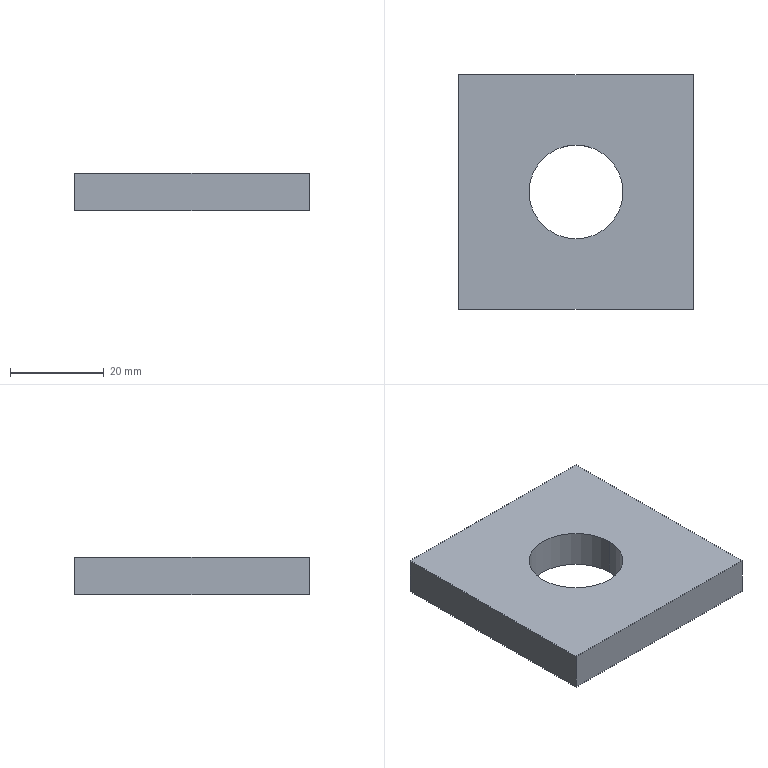Part | STEP file | 立柱底Plate方形垫片 | 1 solid | 8 faces | box 50 x 50 x 8 mm | volume 17487 mm3 | plane 6 | cylinder 2 | commonest cylinder face diameters 20 x2
STEP:
#1=CARTESIAN_POINT('',(0.,0.,0.));
#2=DIRECTION('',(0.,0.,1.));
#3=DIRECTION('',(1.,0.,0.));
#4=AXIS2_PLACEMENT_3D('',#1,#2,#3);
#5=CARTESIAN_POINT('',(-10.,0.,8.));
#6=VERTEX_POINT('',#5);
#7=CARTESIAN_POINT('',(-10.,0.,0.));
#8=VERTEX_POINT('',#7);
#9=CARTESIAN_POINT('',(-10.,0.,8.));
#10=DIRECTION('',(0.,0.,-1.));
#11=VECTOR('',#10,1.);
#12=LINE('',#9,#11);
#13=CARTESIAN_POINT('',(0.,0.,8.));
#14=DIRECTION('',(0.,0.,-1.));
#15=DIRECTION('',(-1.,0.,0.));
#16=AXIS2_PLACEMENT_3D('',#13,#14,#15);
#17=CYLINDRICAL_SURFACE('',#16,10.);
#18=CARTESIAN_POINT('',(6.283,0.));
#19=DIRECTION('',(0.,1.));
#20=VECTOR('',#19,1.);
#21=LINE('',#18,#20);
#22=(GEOMETRIC_REPRESENTATION_CONTEXT(2)PARAMETRIC_REPRESENTATION_CONTEXT()REPRESENTATION_CONTEXT('',''));
#23=DEFINITIONAL_REPRESENTATION('',(#21),#22);
#24=PCURVE('',#17,#23);
#25=CARTESIAN_POINT('',(0.,0.,8.));
#26=DIRECTION('',(0.,0.,-1.));
#27=DIRECTION('',(-1.,0.,0.));
#28=AXIS2_PLACEMENT_3D('',#25,#26,#27);
#29=CYLINDRICAL_SURFACE('',#28,10.);
#30=CARTESIAN_POINT('',(0.,0.));
#31=DIRECTION('',(0.,1.));
#32=VECTOR('',#31,1.);
#33=LINE('',#30,#32);
#34=(GEOMETRIC_REPRESENTATION_CONTEXT(2)PARAMETRIC_REPRESENTATION_CONTEXT()REPRESENTATION_CONTEXT('',''));
#35=DEFINITIONAL_REPRESENTATION('',(#33),#34);
#36=PCURVE('',#29,#35);
#37=SURFACE_CURVE('',#12,(#24,#36),.PCURVE_S1.);
#38=EDGE_CURVE('',#6,#8,#37,.T.);
#39=ORIENTED_EDGE('',*,*,#38,.T.);
#40=CARTESIAN_POINT('',(10.,0.,0.));
#41=VERTEX_POINT('',#40);
#42=CARTESIAN_POINT('',(0.,0.,0.));
#43=DIRECTION('',(0.,0.,1.));
#44=DIRECTION('',(1.,0.,0.));
#45=AXIS2_PLACEMENT_3D('',#42,#43,#44);
#46=CIRCLE('',#45,10.);
#47=CARTESIAN_POINT('',(9.425,8.));
#48=DIRECTION('',(-1.,0.));
#49=VECTOR('',#48,1.);
#50=LINE('',#47,#49);
#51=(GEOMETRIC_REPRESENTATION_CONTEXT(2)PARAMETRIC_REPRESENTATION_CONTEXT()REPRESENTATION_CONTEXT('',''));
#52=DEFINITIONAL_REPRESENTATION('',(#50),#51);
#53=PCURVE('',#17,#52);
#54=CARTESIAN_POINT('',(0.,0.,0.));
#55=DIRECTION('',(0.,0.,1.));
#56=DIRECTION('',(1.,0.,0.));
#57=AXIS2_PLACEMENT_3D('',#54,#55,#56);
#58=PLANE('',#57);
#59=CARTESIAN_POINT('',(0.,0.));
#60=DIRECTION('',(1.,0.));
#61=AXIS2_PLACEMENT_2D('',#59,#60);
#62=CIRCLE('',#61,10.);
#63=(GEOMETRIC_REPRESENTATION_CONTEXT(2)PARAMETRIC_REPRESENTATION_CONTEXT()REPRESENTATION_CONTEXT('',''));
#64=DEFINITIONAL_REPRESENTATION('',(#62),#63);
#65=PCURVE('',#58,#64);
#66=SURFACE_CURVE('',#46,(#53,#65),.PCURVE_S1.);
#67=EDGE_CURVE('',#8,#41,#66,.T.);
#68=ORIENTED_EDGE('',*,*,#67,.T.);
#69=CARTESIAN_POINT('',(10.,0.,8.));
#70=VERTEX_POINT('',#69);
#71=CARTESIAN_POINT('',(10.,0.,8.));
#72=DIRECTION('',(0.,0.,-1.));
#73=VECTOR('',#72,1.);
#74=LINE('',#71,#73);
#75=CARTESIAN_POINT('',(3.142,0.));
#76=DIRECTION('',(0.,1.));
#77=VECTOR('',#76,1.);
#78=LINE('',#75,#77);
#79=(GEOMETRIC_REPRESENTATION_CONTEXT(2)PARAMETRIC_REPRESENTATION_CONTEXT()REPRESENTATION_CONTEXT('',''));
#80=DEFINITIONAL_REPRESENTATION('',(#78),#79);
#81=PCURVE('',#17,#80);
#82=CARTESIAN_POINT('',(3.142,0.));
#83=DIRECTION('',(0.,1.));
#84=VECTOR('',#83,1.);
#85=LINE('',#82,#84);
#86=(GEOMETRIC_REPRESENTATION_CONTEXT(2)PARAMETRIC_REPRESENTATION_CONTEXT()REPRESENTATION_CONTEXT('',''));
#87=DEFINITIONAL_REPRESENTATION('',(#85),#86);
#88=PCURVE('',#29,#87);
#89=SURFACE_CURVE('',#74,(#81,#88),.PCURVE_S1.);
#90=EDGE_CURVE('',#70,#41,#89,.T.);
#91=ORIENTED_EDGE('',*,*,#90,.F.);
#92=CARTESIAN_POINT('',(0.,0.,8.));
#93=DIRECTION('',(0.,0.,1.));
#94=DIRECTION('',(1.,0.,0.));
#95=AXIS2_PLACEMENT_3D('',#92,#93,#94);
#96=CIRCLE('',#95,10.);
#97=CARTESIAN_POINT('',(9.425,0.));
#98=DIRECTION('',(-1.,0.));
#99=VECTOR('',#98,1.);
#100=LINE('',#97,#99);
#101=(GEOMETRIC_REPRESENTATION_CONTEXT(2)PARAMETRIC_REPRESENTATION_CONTEXT()REPRESENTATION_CONTEXT('',''));
#102=DEFINITIONAL_REPRESENTATION('',(#100),#101);
#103=PCURVE('',#17,#102);
#104=CARTESIAN_POINT('',(0.,0.,8.));
#105=DIRECTION('',(0.,0.,1.));
#106=DIRECTION('',(1.,0.,0.));
#107=AXIS2_PLACEMENT_3D('',#104,#105,#106);
#108=PLANE('',#107);
#109=CARTESIAN_POINT('',(0.,0.));
#110=DIRECTION('',(1.,0.));
#111=AXIS2_PLACEMENT_2D('',#109,#110);
#112=CIRCLE('',#111,10.);
#113=(GEOMETRIC_REPRESENTATION_CONTEXT(2)PARAMETRIC_REPRESENTATION_CONTEXT()REPRESENTATION_CONTEXT('',''));
#114=DEFINITIONAL_REPRESENTATION('',(#112),#113);
#115=PCURVE('',#108,#114);
#116=SURFACE_CURVE('',#96,(#103,#115),.PCURVE_S1.);
#117=EDGE_CURVE('',#6,#70,#116,.T.);
#118=ORIENTED_EDGE('',*,*,#117,.F.);
#119=EDGE_LOOP('',(#39,#68,#91,#118));
#120=FACE_BOUND('',#119,.F.);
#121=ADVANCED_FACE('',(#120),#17,.F.);
#122=CARTESIAN_POINT('',(25.,-25.,8.));
#123=VERTEX_POINT('',#122);
#124=CARTESIAN_POINT('',(25.,25.,8.));
#125=VERTEX_POINT('',#124);
#126=CARTESIAN_POINT('',(25.,25.,8.));
#127=DIRECTION('',(0.,1.,0.));
#128=VECTOR('',#127,1.);
#129=LINE('',#126,#128);
#130=CARTESIAN_POINT('',(25.,25.));
#131=DIRECTION('',(0.,1.));
#132=VECTOR('',#131,1.);
#133=LINE('',#130,#132);
#134=(GEOMETRIC_REPRESENTATION_CONTEXT(2)PARAMETRIC_REPRESENTATION_CONTEXT()REPRESENTATION_CONTEXT('',''));
#135=DEFINITIONAL_REPRESENTATION('',(#133),#134);
#136=PCURVE('',#108,#135);
#137=CARTESIAN_POINT('',(25.,25.,8.));
#138=DIRECTION('',(-1.,0.,0.));
#139=DIRECTION('',(0.,-1.,0.));
#140=AXIS2_PLACEMENT_3D('',#137,#138,#139);
#141=PLANE('',#140);
#142=CARTESIAN_POINT('',(0.,0.));
#143=DIRECTION('',(-1.,0.));
#144=VECTOR('',#143,1.);
#145=LINE('',#142,#144);
#146=(GEOMETRIC_REPRESENTATION_CONTEXT(2)PARAMETRIC_REPRESENTATION_CONTEXT()REPRESENTATION_CONTEXT('',''));
#147=DEFINITIONAL_REPRESENTATION('',(#145),#146);
#148=PCURVE('',#141,#147);
#149=SURFACE_CURVE('',#129,(#136,#148),.PCURVE_S1.);
#150=EDGE_CURVE('',#123,#125,#149,.T.);
#151=ORIENTED_EDGE('',*,*,#150,.T.);
#152=CARTESIAN_POINT('',(-25.,25.,8.));
#153=VERTEX_POINT('',#152);
#154=CARTESIAN_POINT('',(-25.,25.,8.));
#155=DIRECTION('',(-1.,0.,0.));
#156=VECTOR('',#155,1.);
#157=LINE('',#154,#156);
#158=CARTESIAN_POINT('',(-25.,25.));
#159=DIRECTION('',(-1.,0.));
#160=VECTOR('',#159,1.);
#161=LINE('',#158,#160);
#162=(GEOMETRIC_REPRESENTATION_CONTEXT(2)PARAMETRIC_REPRESENTATION_CONTEXT()REPRESENTATION_CONTEXT('',''));
#163=DEFINITIONAL_REPRESENTATION('',(#161),#162);
#164=PCURVE('',#108,#163);
#165=CARTESIAN_POINT('',(-25.,25.,8.));
#166=DIRECTION('',(0.,-1.,0.));
#167=DIRECTION('',(0.,0.,-1.));
#168=AXIS2_PLACEMENT_3D('',#165,#166,#167);
#169=PLANE('',#168);
#170=CARTESIAN_POINT('',(0.,0.));
#171=DIRECTION('',(0.,-1.));
#172=VECTOR('',#171,1.);
#173=LINE('',#170,#172);
#174=(GEOMETRIC_REPRESENTATION_CONTEXT(2)PARAMETRIC_REPRESENTATION_CONTEXT()REPRESENTATION_CONTEXT('',''));
#175=DEFINITIONAL_REPRESENTATION('',(#173),#174);
#176=PCURVE('',#169,#175);
#177=SURFACE_CURVE('',#157,(#164,#176),.PCURVE_S1.);
#178=EDGE_CURVE('',#125,#153,#177,.T.);
#179=ORIENTED_EDGE('',*,*,#178,.T.);
#180=CARTESIAN_POINT('',(-25.,-25.,8.));
#181=VERTEX_POINT('',#180);
#182=CARTESIAN_POINT('',(-25.,25.,8.));
#183=DIRECTION('',(0.,-1.,0.));
#184=VECTOR('',#183,1.);
#185=LINE('',#182,#184);
#186=CARTESIAN_POINT('',(-25.,25.));
#187=DIRECTION('',(0.,-1.));
#188=VECTOR('',#187,1.);
#189=LINE('',#186,#188);
#190=(GEOMETRIC_REPRESENTATION_CONTEXT(2)PARAMETRIC_REPRESENTATION_CONTEXT()REPRESENTATION_CONTEXT('',''));
#191=DEFINITIONAL_REPRESENTATION('',(#189),#190);
#192=PCURVE('',#108,#191);
#193=CARTESIAN_POINT('',(-25.,25.,8.));
#194=DIRECTION('',(1.,0.,0.));
#195=DIRECTION('',(0.,1.,0.));
#196=AXIS2_PLACEMENT_3D('',#193,#194,#195);
#197=PLANE('',#196);
#198=CARTESIAN_POINT('',(0.,0.));
#199=DIRECTION('',(-1.,0.));
#200=VECTOR('',#199,1.);
#201=LINE('',#198,#200);
#202=(GEOMETRIC_REPRESENTATION_CONTEXT(2)PARAMETRIC_REPRESENTATION_CONTEXT()REPRESENTATION_CONTEXT('',''));
#203=DEFINITIONAL_REPRESENTATION('',(#201),#202);
#204=PCURVE('',#197,#203);
#205=SURFACE_CURVE('',#185,(#192,#204),.PCURVE_S1.);
#206=EDGE_CURVE('',#153,#181,#205,.T.);
#207=ORIENTED_EDGE('',*,*,#206,.T.);
#208=CARTESIAN_POINT('',(-25.,-25.,8.));
#209=DIRECTION('',(1.,0.,0.));
#210=VECTOR('',#209,1.);
#211=LINE('',#208,#210);
#212=CARTESIAN_POINT('',(-25.,-25.));
#213=DIRECTION('',(1.,0.));
#214=VECTOR('',#213,1.);
#215=LINE('',#212,#214);
#216=(GEOMETRIC_REPRESENTATION_CONTEXT(2)PARAMETRIC_REPRESENTATION_CONTEXT()REPRESENTATION_CONTEXT('',''));
#217=DEFINITIONAL_REPRESENTATION('',(#215),#216);
#218=PCURVE('',#108,#217);
#219=CARTESIAN_POINT('',(-25.,-25.,8.));
#220=DIRECTION('',(0.,1.,0.));
#221=DIRECTION('',(0.,0.,1.));
#222=AXIS2_PLACEMENT_3D('',#219,#220,#221);
#223=PLANE('',#222);
#224=CARTESIAN_POINT('',(0.,0.));
#225=DIRECTION('',(0.,1.));
#226=VECTOR('',#225,1.);
#227=LINE('',#224,#226);
#228=(GEOMETRIC_REPRESENTATION_CONTEXT(2)PARAMETRIC_REPRESENTATION_CONTEXT()REPRESENTATION_CONTEXT('',''));
#229=DEFINITIONAL_REPRESENTATION('',(#227),#228);
#230=PCURVE('',#223,#229);
#231=SURFACE_CURVE('',#211,(#218,#230),.PCURVE_S1.);
#232=EDGE_CURVE('',#181,#123,#231,.T.);
#233=ORIENTED_EDGE('',*,*,#232,.T.);
#234=EDGE_LOOP('',(#151,#179,#207,#233));
#235=FACE_BOUND('',#234,.T.);
#236=ORIENTED_EDGE('',*,*,#117,.F.);
#237=CARTESIAN_POINT('',(0.,0.,8.));
#238=DIRECTION('',(0.,0.,1.));
#239=DIRECTION('',(1.,0.,0.));
#240=AXIS2_PLACEMENT_3D('',#237,#238,#239);
#241=CIRCLE('',#240,10.);
#242=CARTESIAN_POINT('',(0.,0.));
#243=DIRECTION('',(1.,0.));
#244=AXIS2_PLACEMENT_2D('',#242,#243);
#245=CIRCLE('',#244,10.);
#246=(GEOMETRIC_REPRESENTATION_CONTEXT(2)PARAMETRIC_REPRESENTATION_CONTEXT()REPRESENTATION_CONTEXT('',''));
#247=DEFINITIONAL_REPRESENTATION('',(#245),#246);
#248=PCURVE('',#108,#247);
#249=CARTESIAN_POINT('',(3.142,0.));
#250=DIRECTION('',(-1.,0.));
#251=VECTOR('',#250,1.);
#252=LINE('',#249,#251);
#253=(GEOMETRIC_REPRESENTATION_CONTEXT(2)PARAMETRIC_REPRESENTATION_CONTEXT()REPRESENTATION_CONTEXT('',''));
#254=DEFINITIONAL_REPRESENTATION('',(#252),#253);
#255=PCURVE('',#29,#254);
#256=SURFACE_CURVE('',#241,(#248,#255),.PCURVE_S1.);
#257=EDGE_CURVE('',#70,#6,#256,.T.);
#258=ORIENTED_EDGE('',*,*,#257,.F.);
#259=EDGE_LOOP('',(#236,#258));
#260=FACE_BOUND('',#259,.T.);
#261=ADVANCED_FACE('',(#235,#260),#108,.T.);
#262=CARTESIAN_POINT('',(25.,-25.,0.));
#263=VERTEX_POINT('',#262);
#264=CARTESIAN_POINT('',(25.,25.,0.));
#265=VERTEX_POINT('',#264);
#266=CARTESIAN_POINT('',(25.,25.,0.));
#267=DIRECTION('',(0.,1.,0.));
#268=VECTOR('',#267,1.);
#269=LINE('',#266,#268);
#270=CARTESIAN_POINT('',(25.,25.));
#271=DIRECTION('',(0.,1.));
#272=VECTOR('',#271,1.);
#273=LINE('',#270,#272);
#274=(GEOMETRIC_REPRESENTATION_CONTEXT(2)PARAMETRIC_REPRESENTATION_CONTEXT()REPRESENTATION_CONTEXT('',''));
#275=DEFINITIONAL_REPRESENTATION('',(#273),#274);
#276=PCURVE('',#58,#275);
#277=CARTESIAN_POINT('',(0.,-8.));
#278=DIRECTION('',(-1.,0.));
#279=VECTOR('',#278,1.);
#280=LINE('',#277,#279);
#281=(GEOMETRIC_REPRESENTATION_CONTEXT(2)PARAMETRIC_REPRESENTATION_CONTEXT()REPRESENTATION_CONTEXT('',''));
#282=DEFINITIONAL_REPRESENTATION('',(#280),#281);
#283=PCURVE('',#141,#282);
#284=SURFACE_CURVE('',#269,(#276,#283),.PCURVE_S1.);
#285=EDGE_CURVE('',#263,#265,#284,.T.);
#286=ORIENTED_EDGE('',*,*,#285,.F.);
#287=CARTESIAN_POINT('',(-25.,-25.,0.));
#288=VERTEX_POINT('',#287);
#289=CARTESIAN_POINT('',(-25.,-25.,0.));
#290=DIRECTION('',(1.,0.,0.));
#291=VECTOR('',#290,1.);
#292=LINE('',#289,#291);
#293=CARTESIAN_POINT('',(-25.,-25.));
#294=DIRECTION('',(1.,0.));
#295=VECTOR('',#294,1.);
#296=LINE('',#293,#295);
#297=(GEOMETRIC_REPRESENTATION_CONTEXT(2)PARAMETRIC_REPRESENTATION_CONTEXT()REPRESENTATION_CONTEXT('',''));
#298=DEFINITIONAL_REPRESENTATION('',(#296),#297);
#299=PCURVE('',#58,#298);
#300=CARTESIAN_POINT('',(-8.,0.));
#301=DIRECTION('',(0.,1.));
#302=VECTOR('',#301,1.);
#303=LINE('',#300,#302);
#304=(GEOMETRIC_REPRESENTATION_CONTEXT(2)PARAMETRIC_REPRESENTATION_CONTEXT()REPRESENTATION_CONTEXT('',''));
#305=DEFINITIONAL_REPRESENTATION('',(#303),#304);
#306=PCURVE('',#223,#305);
#307=SURFACE_CURVE('',#292,(#299,#306),.PCURVE_S1.);
#308=EDGE_CURVE('',#288,#263,#307,.T.);
#309=ORIENTED_EDGE('',*,*,#308,.F.);
#310=CARTESIAN_POINT('',(-25.,25.,0.));
#311=VERTEX_POINT('',#310);
#312=CARTESIAN_POINT('',(-25.,25.,0.));
#313=DIRECTION('',(0.,-1.,0.));
#314=VECTOR('',#313,1.);
#315=LINE('',#312,#314);
#316=CARTESIAN_POINT('',(-25.,25.));
#317=DIRECTION('',(0.,-1.));
#318=VECTOR('',#317,1.);
#319=LINE('',#316,#318);
#320=(GEOMETRIC_REPRESENTATION_CONTEXT(2)PARAMETRIC_REPRESENTATION_CONTEXT()REPRESENTATION_CONTEXT('',''));
#321=DEFINITIONAL_REPRESENTATION('',(#319),#320);
#322=PCURVE('',#58,#321);
#323=CARTESIAN_POINT('',(0.,-8.));
#324=DIRECTION('',(-1.,0.));
#325=VECTOR('',#324,1.);
#326=LINE('',#323,#325);
#327=(GEOMETRIC_REPRESENTATION_CONTEXT(2)PARAMETRIC_REPRESENTATION_CONTEXT()REPRESENTATION_CONTEXT('',''));
#328=DEFINITIONAL_REPRESENTATION('',(#326),#327);
#329=PCURVE('',#197,#328);
#330=SURFACE_CURVE('',#315,(#322,#329),.PCURVE_S1.);
#331=EDGE_CURVE('',#311,#288,#330,.T.);
#332=ORIENTED_EDGE('',*,*,#331,.F.);
#333=CARTESIAN_POINT('',(-25.,25.,0.));
#334=DIRECTION('',(-1.,0.,0.));
#335=VECTOR('',#334,1.);
#336=LINE('',#333,#335);
#337=CARTESIAN_POINT('',(-25.,25.));
#338=DIRECTION('',(-1.,0.));
#339=VECTOR('',#338,1.);
#340=LINE('',#337,#339);
#341=(GEOMETRIC_REPRESENTATION_CONTEXT(2)PARAMETRIC_REPRESENTATION_CONTEXT()REPRESENTATION_CONTEXT('',''));
#342=DEFINITIONAL_REPRESENTATION('',(#340),#341);
#343=PCURVE('',#58,#342);
#344=CARTESIAN_POINT('',(8.,0.));
#345=DIRECTION('',(0.,-1.));
#346=VECTOR('',#345,1.);
#347=LINE('',#344,#346);
#348=(GEOMETRIC_REPRESENTATION_CONTEXT(2)PARAMETRIC_REPRESENTATION_CONTEXT()REPRESENTATION_CONTEXT('',''));
#349=DEFINITIONAL_REPRESENTATION('',(#347),#348);
#350=PCURVE('',#169,#349);
#351=SURFACE_CURVE('',#336,(#343,#350),.PCURVE_S1.);
#352=EDGE_CURVE('',#265,#311,#351,.T.);
#353=ORIENTED_EDGE('',*,*,#352,.F.);
#354=EDGE_LOOP('',(#286,#309,#332,#353));
#355=FACE_BOUND('',#354,.T.);
#356=ORIENTED_EDGE('',*,*,#67,.T.);
#357=CARTESIAN_POINT('',(0.,0.,0.));
#358=DIRECTION('',(0.,0.,1.));
#359=DIRECTION('',(1.,0.,0.));
#360=AXIS2_PLACEMENT_3D('',#357,#358,#359);
#361=CIRCLE('',#360,10.);
#362=CARTESIAN_POINT('',(0.,0.));
#363=DIRECTION('',(1.,0.));
#364=AXIS2_PLACEMENT_2D('',#362,#363);
#365=CIRCLE('',#364,10.);
#366=(GEOMETRIC_REPRESENTATION_CONTEXT(2)PARAMETRIC_REPRESENTATION_CONTEXT()REPRESENTATION_CONTEXT('',''));
#367=DEFINITIONAL_REPRESENTATION('',(#365),#366);
#368=PCURVE('',#58,#367);
#369=CARTESIAN_POINT('',(3.142,8.));
#370=DIRECTION('',(-1.,0.));
#371=VECTOR('',#370,1.);
#372=LINE('',#369,#371);
#373=(GEOMETRIC_REPRESENTATION_CONTEXT(2)PARAMETRIC_REPRESENTATION_CONTEXT()REPRESENTATION_CONTEXT('',''));
#374=DEFINITIONAL_REPRESENTATION('',(#372),#373);
#375=PCURVE('',#29,#374);
#376=SURFACE_CURVE('',#361,(#368,#375),.PCURVE_S1.);
#377=EDGE_CURVE('',#41,#8,#376,.T.);
#378=ORIENTED_EDGE('',*,*,#377,.T.);
#379=EDGE_LOOP('',(#356,#378));
#380=FACE_BOUND('',#379,.T.);
#381=ADVANCED_FACE('',(#355,#380),#58,.F.);
#382=ORIENTED_EDGE('',*,*,#285,.T.);
#383=CARTESIAN_POINT('',(25.,25.,8.));
#384=DIRECTION('',(0.,0.,-1.));
#385=VECTOR('',#384,1.);
#386=LINE('',#383,#385);
#387=CARTESIAN_POINT('',(0.,0.));
#388=DIRECTION('',(0.,-1.));
#389=VECTOR('',#388,1.);
#390=LINE('',#387,#389);
#391=(GEOMETRIC_REPRESENTATION_CONTEXT(2)PARAMETRIC_REPRESENTATION_CONTEXT()REPRESENTATION_CONTEXT('',''));
#392=DEFINITIONAL_REPRESENTATION('',(#390),#391);
#393=PCURVE('',#141,#392);
#394=CARTESIAN_POINT('',(0.,50.));
#395=DIRECTION('',(1.,0.));
#396=VECTOR('',#395,1.);
#397=LINE('',#394,#396);
#398=(GEOMETRIC_REPRESENTATION_CONTEXT(2)PARAMETRIC_REPRESENTATION_CONTEXT()REPRESENTATION_CONTEXT('',''));
#399=DEFINITIONAL_REPRESENTATION('',(#397),#398);
#400=PCURVE('',#169,#399);
#401=SURFACE_CURVE('',#386,(#393,#400),.PCURVE_S1.);
#402=EDGE_CURVE('',#125,#265,#401,.T.);
#403=ORIENTED_EDGE('',*,*,#402,.F.);
#404=ORIENTED_EDGE('',*,*,#150,.F.);
#405=CARTESIAN_POINT('',(25.,-25.,8.));
#406=DIRECTION('',(0.,0.,-1.));
#407=VECTOR('',#406,1.);
#408=LINE('',#405,#407);
#409=CARTESIAN_POINT('',(50.,0.));
#410=DIRECTION('',(0.,-1.));
#411=VECTOR('',#410,1.);
#412=LINE('',#409,#411);
#413=(GEOMETRIC_REPRESENTATION_CONTEXT(2)PARAMETRIC_REPRESENTATION_CONTEXT()REPRESENTATION_CONTEXT('',''));
#414=DEFINITIONAL_REPRESENTATION('',(#412),#413);
#415=PCURVE('',#141,#414);
#416=CARTESIAN_POINT('',(0.,50.));
#417=DIRECTION('',(-1.,0.));
#418=VECTOR('',#417,1.);
#419=LINE('',#416,#418);
#420=(GEOMETRIC_REPRESENTATION_CONTEXT(2)PARAMETRIC_REPRESENTATION_CONTEXT()REPRESENTATION_CONTEXT('',''));
#421=DEFINITIONAL_REPRESENTATION('',(#419),#420);
#422=PCURVE('',#223,#421);
#423=SURFACE_CURVE('',#408,(#415,#422),.PCURVE_S1.);
#424=EDGE_CURVE('',#123,#263,#423,.T.);
#425=ORIENTED_EDGE('',*,*,#424,.T.);
#426=EDGE_LOOP('',(#382,#403,#404,#425));
#427=FACE_BOUND('',#426,.T.);
#428=ADVANCED_FACE('',(#427),#141,.F.);
#429=ORIENTED_EDGE('',*,*,#352,.T.);
#430=CARTESIAN_POINT('',(-25.,25.,8.));
#431=DIRECTION('',(0.,0.,-1.));
#432=VECTOR('',#431,1.);
#433=LINE('',#430,#432);
#434=CARTESIAN_POINT('',(0.,0.));
#435=DIRECTION('',(1.,0.));
#436=VECTOR('',#435,1.);
#437=LINE('',#434,#436);
#438=(GEOMETRIC_REPRESENTATION_CONTEXT(2)PARAMETRIC_REPRESENTATION_CONTEXT()REPRESENTATION_CONTEXT('',''));
#439=DEFINITIONAL_REPRESENTATION('',(#437),#438);
#440=PCURVE('',#169,#439);
#441=CARTESIAN_POINT('',(0.,0.));
#442=DIRECTION('',(0.,-1.));
#443=VECTOR('',#442,1.);
#444=LINE('',#441,#443);
#445=(GEOMETRIC_REPRESENTATION_CONTEXT(2)PARAMETRIC_REPRESENTATION_CONTEXT()REPRESENTATION_CONTEXT('',''));
#446=DEFINITIONAL_REPRESENTATION('',(#444),#445);
#447=PCURVE('',#197,#446);
#448=SURFACE_CURVE('',#433,(#440,#447),.PCURVE_S1.);
#449=EDGE_CURVE('',#153,#311,#448,.T.);
#450=ORIENTED_EDGE('',*,*,#449,.F.);
#451=ORIENTED_EDGE('',*,*,#178,.F.);
#452=ORIENTED_EDGE('',*,*,#402,.T.);
#453=EDGE_LOOP('',(#429,#450,#451,#452));
#454=FACE_BOUND('',#453,.T.);
#455=ADVANCED_FACE('',(#454),#169,.F.);
#456=ORIENTED_EDGE('',*,*,#331,.T.);
#457=CARTESIAN_POINT('',(-25.,-25.,8.));
#458=DIRECTION('',(0.,0.,-1.));
#459=VECTOR('',#458,1.);
#460=LINE('',#457,#459);
#461=CARTESIAN_POINT('',(-50.,0.));
#462=DIRECTION('',(0.,-1.));
#463=VECTOR('',#462,1.);
#464=LINE('',#461,#463);
#465=(GEOMETRIC_REPRESENTATION_CONTEXT(2)PARAMETRIC_REPRESENTATION_CONTEXT()REPRESENTATION_CONTEXT('',''));
#466=DEFINITIONAL_REPRESENTATION('',(#464),#465);
#467=PCURVE('',#197,#466);
#468=CARTESIAN_POINT('',(0.,0.));
#469=DIRECTION('',(-1.,0.));
#470=VECTOR('',#469,1.);
#471=LINE('',#468,#470);
#472=(GEOMETRIC_REPRESENTATION_CONTEXT(2)PARAMETRIC_REPRESENTATION_CONTEXT()REPRESENTATION_CONTEXT('',''));
#473=DEFINITIONAL_REPRESENTATION('',(#471),#472);
#474=PCURVE('',#223,#473);
#475=SURFACE_CURVE('',#460,(#467,#474),.PCURVE_S1.);
#476=EDGE_CURVE('',#181,#288,#475,.T.);
#477=ORIENTED_EDGE('',*,*,#476,.F.);
#478=ORIENTED_EDGE('',*,*,#206,.F.);
#479=ORIENTED_EDGE('',*,*,#449,.T.);
#480=EDGE_LOOP('',(#456,#477,#478,#479));
#481=FACE_BOUND('',#480,.T.);
#482=ADVANCED_FACE('',(#481),#197,.F.);
#483=ORIENTED_EDGE('',*,*,#308,.T.);
#484=ORIENTED_EDGE('',*,*,#424,.F.);
#485=ORIENTED_EDGE('',*,*,#232,.F.);
#486=ORIENTED_EDGE('',*,*,#476,.T.);
#487=EDGE_LOOP('',(#483,#484,#485,#486));
#488=FACE_BOUND('',#487,.T.);
#489=ADVANCED_FACE('',(#488),#223,.F.);
#490=ORIENTED_EDGE('',*,*,#377,.T.);
#491=ORIENTED_EDGE('',*,*,#38,.F.);
#492=ORIENTED_EDGE('',*,*,#257,.F.);
#493=ORIENTED_EDGE('',*,*,#90,.T.);
#494=EDGE_LOOP('',(#490,#491,#492,#493));
#495=FACE_BOUND('',#494,.F.);
#496=ADVANCED_FACE('',(#495),#29,.F.);
#497=CLOSED_SHELL('',(#121,#261,#381,#428,#455,#482,#489,#496));
#498=MANIFOLD_SOLID_BREP('',#497);
#499=(LENGTH_UNIT()NAMED_UNIT(*)SI_UNIT(.MILLI.,.METRE.));
#500=UNCERTAINTY_MEASURE_WITH_UNIT(LENGTH_MEASURE(0.0000001),#499,'','');
#501=(NAMED_UNIT(*)PLANE_ANGLE_UNIT()SI_UNIT($,.RADIAN.));
#502=(NAMED_UNIT(*)SI_UNIT($,.STERADIAN.)SOLID_ANGLE_UNIT());
#503=(GEOMETRIC_REPRESENTATION_CONTEXT(3)GLOBAL_UNCERTAINTY_ASSIGNED_CONTEXT((#500))GLOBAL_UNIT_ASSIGNED_CONTEXT((#499,#501,#502))REPRESENTATION_CONTEXT('',''));
#504=ADVANCED_BREP_SHAPE_REPRESENTATION('',(#4,#498),#503);